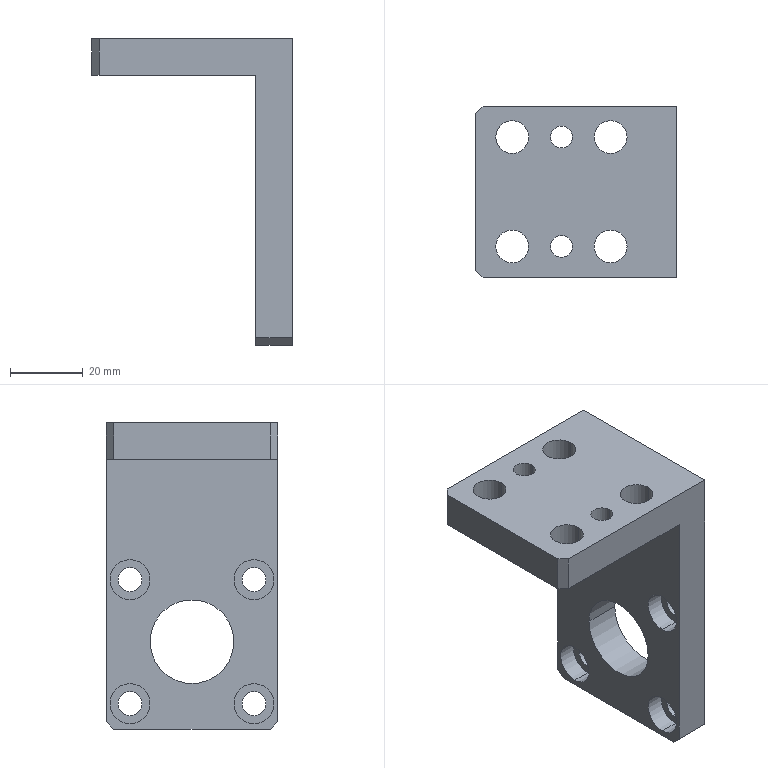Part | SolidWorks | features HoleWzd 3, Chamfer 2, ICE 2, CirPattern 1, Extrusion 1 | 1 solid | 46 faces | box 55 x 47 x 84 mm | volume 50700 mm3 | cylinder 30 | plane 16 | commonest cylinder face diameters 6.6 x8 9 x8 11 x8 6 x4 23 x2
STEP:
#1=CARTESIAN_POINT('',(22.5,-17.,-38.5));
#2=VERTEX_POINT('',#1);
#3=CARTESIAN_POINT('',(22.5,-17.,-27.5));
#4=VERTEX_POINT('',#3);
#5=CARTESIAN_POINT('',(22.5,-17.,-33.));
#6=DIRECTION('',(-1.,0.,0.));
#7=DIRECTION('',(0.,0.,1.));
#8=AXIS2_PLACEMENT_3D('',#5,#6,#7);
#9=CIRCLE('',#8,5.5);
#10=EDGE_CURVE('',#2,#4,#9,.T.);
#11=ORIENTED_EDGE('',*,*,#10,.F.);
#12=CARTESIAN_POINT('',(17.5,-17.,-38.5));
#13=VERTEX_POINT('',#12);
#14=CARTESIAN_POINT('',(17.5,-17.,-38.5));
#15=DIRECTION('',(-1.,0.,0.));
#16=VECTOR('',#15,1000.);
#17=LINE('',#14,#16);
#18=EDGE_CURVE('',#2,#13,#17,.T.);
#19=ORIENTED_EDGE('',*,*,#18,.T.);
#20=CARTESIAN_POINT('',(17.5,-17.,-27.5));
#21=VERTEX_POINT('',#20);
#22=CARTESIAN_POINT('',(17.5,-17.,-33.));
#23=DIRECTION('',(-1.,0.,0.));
#24=DIRECTION('',(0.,0.,1.));
#25=AXIS2_PLACEMENT_3D('',#22,#23,#24);
#26=CIRCLE('',#25,5.5);
#27=EDGE_CURVE('',#13,#21,#26,.T.);
#28=ORIENTED_EDGE('',*,*,#27,.T.);
#29=CARTESIAN_POINT('',(17.5,-17.,-27.5));
#30=DIRECTION('',(-1.,0.,0.));
#31=VECTOR('',#30,1000.);
#32=LINE('',#29,#31);
#33=EDGE_CURVE('',#4,#21,#32,.T.);
#34=ORIENTED_EDGE('',*,*,#33,.F.);
#35=EDGE_LOOP('',(#11,#19,#28,#34));
#36=FACE_OUTER_BOUND('',#35,.T.);
#37=CARTESIAN_POINT('',(17.5,-17.,-33.));
#38=DIRECTION('',(-1.,0.,0.));
#39=DIRECTION('',(0.,0.,1.));
#40=AXIS2_PLACEMENT_3D('',#37,#38,#39);
#41=CYLINDRICAL_SURFACE('',#40,5.5);
#42=ADVANCED_FACE('',(#36),#41,.F.);
#43=CARTESIAN_POINT('',(27.5,-17.,-36.3));
#44=VERTEX_POINT('',#43);
#45=CARTESIAN_POINT('',(27.5,-17.,-29.7));
#46=VERTEX_POINT('',#45);
#47=CARTESIAN_POINT('',(27.5,-17.,-33.));
#48=DIRECTION('',(-1.,0.,0.));
#49=DIRECTION('',(0.,-1.,0.));
#50=AXIS2_PLACEMENT_3D('',#47,#48,#49);
#51=CIRCLE('',#50,3.3);
#52=EDGE_CURVE('',#44,#46,#51,.T.);
#53=ORIENTED_EDGE('',*,*,#52,.F.);
#54=CARTESIAN_POINT('',(22.5,-17.,-36.3));
#55=VERTEX_POINT('',#54);
#56=CARTESIAN_POINT('',(17.5,-17.,-36.3));
#57=DIRECTION('',(-1.,0.,0.));
#58=VECTOR('',#57,1000.);
#59=LINE('',#56,#58);
#60=EDGE_CURVE('',#44,#55,#59,.T.);
#61=ORIENTED_EDGE('',*,*,#60,.T.);
#62=CARTESIAN_POINT('',(22.5,-17.,-29.7));
#63=VERTEX_POINT('',#62);
#64=CARTESIAN_POINT('',(22.5,-17.,-33.));
#65=DIRECTION('',(-1.,0.,0.));
#66=DIRECTION('',(0.,0.,1.));
#67=AXIS2_PLACEMENT_3D('',#64,#65,#66);
#68=CIRCLE('',#67,3.3);
#69=EDGE_CURVE('',#55,#63,#68,.T.);
#70=ORIENTED_EDGE('',*,*,#69,.T.);
#71=CARTESIAN_POINT('',(17.5,-17.,-29.7));
#72=DIRECTION('',(-1.,0.,0.));
#73=VECTOR('',#72,1000.);
#74=LINE('',#71,#73);
#75=EDGE_CURVE('',#46,#63,#74,.T.);
#76=ORIENTED_EDGE('',*,*,#75,.F.);
#77=EDGE_LOOP('',(#53,#61,#70,#76));
#78=FACE_OUTER_BOUND('',#77,.T.);
#79=CARTESIAN_POINT('',(17.5,-17.,-33.));
#80=DIRECTION('',(-1.,0.,0.));
#81=DIRECTION('',(0.,0.,1.));
#82=AXIS2_PLACEMENT_3D('',#79,#80,#81);
#83=CYLINDRICAL_SURFACE('',#82,3.3);
#84=ADVANCED_FACE('',(#78),#83,.F.);
#85=CARTESIAN_POINT('',(22.5,17.,-38.5));
#86=VERTEX_POINT('',#85);
#87=CARTESIAN_POINT('',(22.5,17.,-27.5));
#88=VERTEX_POINT('',#87);
#89=CARTESIAN_POINT('',(22.5,17.,-33.));
#90=DIRECTION('',(-1.,0.,0.));
#91=DIRECTION('',(0.,0.,1.));
#92=AXIS2_PLACEMENT_3D('',#89,#90,#91);
#93=CIRCLE('',#92,5.5);
#94=EDGE_CURVE('',#86,#88,#93,.T.);
#95=ORIENTED_EDGE('',*,*,#94,.F.);
#96=CARTESIAN_POINT('',(17.5,17.,-38.5));
#97=VERTEX_POINT('',#96);
#98=CARTESIAN_POINT('',(17.5,17.,-38.5));
#99=DIRECTION('',(-1.,0.,0.));
#100=VECTOR('',#99,1000.);
#101=LINE('',#98,#100);
#102=EDGE_CURVE('',#86,#97,#101,.T.);
#103=ORIENTED_EDGE('',*,*,#102,.T.);
#104=CARTESIAN_POINT('',(17.5,17.,-27.5));
#105=VERTEX_POINT('',#104);
#106=CARTESIAN_POINT('',(17.5,17.,-33.));
#107=DIRECTION('',(-1.,0.,0.));
#108=DIRECTION('',(0.,0.,1.));
#109=AXIS2_PLACEMENT_3D('',#106,#107,#108);
#110=CIRCLE('',#109,5.5);
#111=EDGE_CURVE('',#97,#105,#110,.T.);
#112=ORIENTED_EDGE('',*,*,#111,.T.);
#113=CARTESIAN_POINT('',(17.5,17.,-27.5));
#114=DIRECTION('',(-1.,0.,0.));
#115=VECTOR('',#114,1000.);
#116=LINE('',#113,#115);
#117=EDGE_CURVE('',#88,#105,#116,.T.);
#118=ORIENTED_EDGE('',*,*,#117,.F.);
#119=EDGE_LOOP('',(#95,#103,#112,#118));
#120=FACE_OUTER_BOUND('',#119,.T.);
#121=CARTESIAN_POINT('',(17.5,17.,-33.));
#122=DIRECTION('',(-1.,0.,0.));
#123=DIRECTION('',(0.,0.,1.));
#124=AXIS2_PLACEMENT_3D('',#121,#122,#123);
#125=CYLINDRICAL_SURFACE('',#124,5.5);
#126=ADVANCED_FACE('',(#120),#125,.F.);
#127=CARTESIAN_POINT('',(27.5,17.,-36.3));
#128=VERTEX_POINT('',#127);
#129=CARTESIAN_POINT('',(27.5,17.,-29.7));
#130=VERTEX_POINT('',#129);
#131=CARTESIAN_POINT('',(27.5,17.,-33.));
#132=DIRECTION('',(-1.,0.,0.));
#133=DIRECTION('',(0.,-1.,0.));
#134=AXIS2_PLACEMENT_3D('',#131,#132,#133);
#135=CIRCLE('',#134,3.3);
#136=EDGE_CURVE('',#128,#130,#135,.T.);
#137=ORIENTED_EDGE('',*,*,#136,.F.);
#138=CARTESIAN_POINT('',(22.5,17.,-36.3));
#139=VERTEX_POINT('',#138);
#140=CARTESIAN_POINT('',(17.5,17.,-36.3));
#141=DIRECTION('',(-1.,0.,0.));
#142=VECTOR('',#141,1000.);
#143=LINE('',#140,#142);
#144=EDGE_CURVE('',#128,#139,#143,.T.);
#145=ORIENTED_EDGE('',*,*,#144,.T.);
#146=CARTESIAN_POINT('',(22.5,17.,-29.7));
#147=VERTEX_POINT('',#146);
#148=CARTESIAN_POINT('',(22.5,17.,-33.));
#149=DIRECTION('',(-1.,0.,0.));
#150=DIRECTION('',(0.,0.,1.));
#151=AXIS2_PLACEMENT_3D('',#148,#149,#150);
#152=CIRCLE('',#151,3.3);
#153=EDGE_CURVE('',#139,#147,#152,.T.);
#154=ORIENTED_EDGE('',*,*,#153,.T.);
#155=CARTESIAN_POINT('',(17.5,17.,-29.7));
#156=DIRECTION('',(-1.,0.,0.));
#157=VECTOR('',#156,1000.);
#158=LINE('',#155,#157);
#159=EDGE_CURVE('',#130,#147,#158,.T.);
#160=ORIENTED_EDGE('',*,*,#159,.F.);
#161=EDGE_LOOP('',(#137,#145,#154,#160));
#162=FACE_OUTER_BOUND('',#161,.T.);
#163=CARTESIAN_POINT('',(17.5,17.,-33.));
#164=DIRECTION('',(-1.,0.,0.));
#165=DIRECTION('',(0.,0.,1.));
#166=AXIS2_PLACEMENT_3D('',#163,#164,#165);
#167=CYLINDRICAL_SURFACE('',#166,3.3);
#168=ADVANCED_FACE('',(#162),#167,.F.);
#169=CARTESIAN_POINT('',(22.5,17.,-72.5));
#170=VERTEX_POINT('',#169);
#171=CARTESIAN_POINT('',(22.5,17.,-61.5));
#172=VERTEX_POINT('',#171);
#173=CARTESIAN_POINT('',(22.5,17.,-67.));
#174=DIRECTION('',(-1.,0.,0.));
#175=DIRECTION('',(0.,0.,1.));
#176=AXIS2_PLACEMENT_3D('',#173,#174,#175);
#177=CIRCLE('',#176,5.5);
#178=EDGE_CURVE('',#170,#172,#177,.T.);
#179=ORIENTED_EDGE('',*,*,#178,.F.);
#180=CARTESIAN_POINT('',(17.5,17.,-72.5));
#181=VERTEX_POINT('',#180);
#182=CARTESIAN_POINT('',(17.5,17.,-72.5));
#183=DIRECTION('',(-1.,0.,0.));
#184=VECTOR('',#183,1000.);
#185=LINE('',#182,#184);
#186=EDGE_CURVE('',#170,#181,#185,.T.);
#187=ORIENTED_EDGE('',*,*,#186,.T.);
#188=CARTESIAN_POINT('',(17.5,17.,-61.5));
#189=VERTEX_POINT('',#188);
#190=CARTESIAN_POINT('',(17.5,17.,-67.));
#191=DIRECTION('',(-1.,0.,0.));
#192=DIRECTION('',(0.,0.,1.));
#193=AXIS2_PLACEMENT_3D('',#190,#191,#192);
#194=CIRCLE('',#193,5.5);
#195=EDGE_CURVE('',#181,#189,#194,.T.);
#196=ORIENTED_EDGE('',*,*,#195,.T.);
#197=CARTESIAN_POINT('',(17.5,17.,-61.5));
#198=DIRECTION('',(-1.,0.,0.));
#199=VECTOR('',#198,1000.);
#200=LINE('',#197,#199);
#201=EDGE_CURVE('',#172,#189,#200,.T.);
#202=ORIENTED_EDGE('',*,*,#201,.F.);
#203=EDGE_LOOP('',(#179,#187,#196,#202));
#204=FACE_OUTER_BOUND('',#203,.T.);
#205=CARTESIAN_POINT('',(17.5,17.,-67.));
#206=DIRECTION('',(-1.,0.,0.));
#207=DIRECTION('',(0.,0.,1.));
#208=AXIS2_PLACEMENT_3D('',#205,#206,#207);
#209=CYLINDRICAL_SURFACE('',#208,5.5);
#210=ADVANCED_FACE('',(#204),#209,.F.);
#211=CARTESIAN_POINT('',(27.5,17.,-70.3));
#212=VERTEX_POINT('',#211);
#213=CARTESIAN_POINT('',(27.5,17.,-63.7));
#214=VERTEX_POINT('',#213);
#215=CARTESIAN_POINT('',(27.5,17.,-67.));
#216=DIRECTION('',(-1.,0.,0.));
#217=DIRECTION('',(0.,-1.,0.));
#218=AXIS2_PLACEMENT_3D('',#215,#216,#217);
#219=CIRCLE('',#218,3.3);
#220=EDGE_CURVE('',#212,#214,#219,.T.);
#221=ORIENTED_EDGE('',*,*,#220,.F.);
#222=CARTESIAN_POINT('',(22.5,17.,-70.3));
#223=VERTEX_POINT('',#222);
#224=CARTESIAN_POINT('',(17.5,17.,-70.3));
#225=DIRECTION('',(-1.,0.,0.));
#226=VECTOR('',#225,1000.);
#227=LINE('',#224,#226);
#228=EDGE_CURVE('',#212,#223,#227,.T.);
#229=ORIENTED_EDGE('',*,*,#228,.T.);
#230=CARTESIAN_POINT('',(22.5,17.,-63.7));
#231=VERTEX_POINT('',#230);
#232=CARTESIAN_POINT('',(22.5,17.,-67.));
#233=DIRECTION('',(-1.,0.,0.));
#234=DIRECTION('',(0.,0.,1.));
#235=AXIS2_PLACEMENT_3D('',#232,#233,#234);
#236=CIRCLE('',#235,3.3);
#237=EDGE_CURVE('',#223,#231,#236,.T.);
#238=ORIENTED_EDGE('',*,*,#237,.T.);
#239=CARTESIAN_POINT('',(17.5,17.,-63.7));
#240=DIRECTION('',(-1.,0.,0.));
#241=VECTOR('',#240,1000.);
#242=LINE('',#239,#241);
#243=EDGE_CURVE('',#214,#231,#242,.T.);
#244=ORIENTED_EDGE('',*,*,#243,.F.);
#245=EDGE_LOOP('',(#221,#229,#238,#244));
#246=FACE_OUTER_BOUND('',#245,.T.);
#247=CARTESIAN_POINT('',(17.5,17.,-67.));
#248=DIRECTION('',(-1.,0.,0.));
#249=DIRECTION('',(0.,0.,1.));
#250=AXIS2_PLACEMENT_3D('',#247,#248,#249);
#251=CYLINDRICAL_SURFACE('',#250,3.3);
#252=ADVANCED_FACE('',(#246),#251,.F.);
#253=CARTESIAN_POINT('',(22.5,-17.,-72.5));
#254=VERTEX_POINT('',#253);
#255=CARTESIAN_POINT('',(22.5,-17.,-61.5));
#256=VERTEX_POINT('',#255);
#257=CARTESIAN_POINT('',(22.5,-17.,-67.));
#258=DIRECTION('',(-1.,0.,0.));
#259=DIRECTION('',(0.,0.,1.));
#260=AXIS2_PLACEMENT_3D('',#257,#258,#259);
#261=CIRCLE('',#260,5.5);
#262=EDGE_CURVE('',#254,#256,#261,.T.);
#263=ORIENTED_EDGE('',*,*,#262,.F.);
#264=CARTESIAN_POINT('',(17.5,-17.,-72.5));
#265=VERTEX_POINT('',#264);
#266=CARTESIAN_POINT('',(17.5,-17.,-72.5));
#267=DIRECTION('',(-1.,0.,0.));
#268=VECTOR('',#267,1000.);
#269=LINE('',#266,#268);
#270=EDGE_CURVE('',#254,#265,#269,.T.);
#271=ORIENTED_EDGE('',*,*,#270,.T.);
#272=CARTESIAN_POINT('',(17.5,-17.,-61.5));
#273=VERTEX_POINT('',#272);
#274=CARTESIAN_POINT('',(17.5,-17.,-67.));
#275=DIRECTION('',(-1.,0.,0.));
#276=DIRECTION('',(0.,0.,1.));
#277=AXIS2_PLACEMENT_3D('',#274,#275,#276);
#278=CIRCLE('',#277,5.5);
#279=EDGE_CURVE('',#265,#273,#278,.T.);
#280=ORIENTED_EDGE('',*,*,#279,.T.);
#281=CARTESIAN_POINT('',(17.5,-17.,-61.5));
#282=DIRECTION('',(-1.,0.,0.));
#283=VECTOR('',#282,1000.);
#284=LINE('',#281,#283);
#285=EDGE_CURVE('',#256,#273,#284,.T.);
#286=ORIENTED_EDGE('',*,*,#285,.F.);
#287=EDGE_LOOP('',(#263,#271,#280,#286));
#288=FACE_OUTER_BOUND('',#287,.T.);
#289=CARTESIAN_POINT('',(17.5,-17.,-67.));
#290=DIRECTION('',(-1.,0.,0.));
#291=DIRECTION('',(0.,0.,1.));
#292=AXIS2_PLACEMENT_3D('',#289,#290,#291);
#293=CYLINDRICAL_SURFACE('',#292,5.5);
#294=ADVANCED_FACE('',(#288),#293,.F.);
#295=CARTESIAN_POINT('',(27.5,-17.,-70.3));
#296=VERTEX_POINT('',#295);
#297=CARTESIAN_POINT('',(27.5,-17.,-63.7));
#298=VERTEX_POINT('',#297);
#299=CARTESIAN_POINT('',(27.5,-17.,-67.));
#300=DIRECTION('',(-1.,0.,0.));
#301=DIRECTION('',(0.,-1.,0.));
#302=AXIS2_PLACEMENT_3D('',#299,#300,#301);
#303=CIRCLE('',#302,3.3);
#304=EDGE_CURVE('',#296,#298,#303,.T.);
#305=ORIENTED_EDGE('',*,*,#304,.F.);
#306=CARTESIAN_POINT('',(22.5,-17.,-70.3));
#307=VERTEX_POINT('',#306);
#308=CARTESIAN_POINT('',(17.5,-17.,-70.3));
#309=DIRECTION('',(-1.,0.,0.));
#310=VECTOR('',#309,1000.);
#311=LINE('',#308,#310);
#312=EDGE_CURVE('',#296,#307,#311,.T.);
#313=ORIENTED_EDGE('',*,*,#312,.T.);
#314=CARTESIAN_POINT('',(22.5,-17.,-63.7));
#315=VERTEX_POINT('',#314);
#316=CARTESIAN_POINT('',(22.5,-17.,-67.));
#317=DIRECTION('',(-1.,0.,0.));
#318=DIRECTION('',(0.,0.,1.));
#319=AXIS2_PLACEMENT_3D('',#316,#317,#318);
#320=CIRCLE('',#319,3.3);
#321=EDGE_CURVE('',#307,#315,#320,.T.);
#322=ORIENTED_EDGE('',*,*,#321,.T.);
#323=CARTESIAN_POINT('',(17.5,-17.,-63.7));
#324=DIRECTION('',(-1.,0.,0.));
#325=VECTOR('',#324,1000.);
#326=LINE('',#323,#325);
#327=EDGE_CURVE('',#298,#315,#326,.T.);
#328=ORIENTED_EDGE('',*,*,#327,.F.);
#329=EDGE_LOOP('',(#305,#313,#322,#328));
#330=FACE_OUTER_BOUND('',#329,.T.);
#331=CARTESIAN_POINT('',(17.5,-17.,-67.));
#332=DIRECTION('',(-1.,0.,0.));
#333=DIRECTION('',(0.,0.,1.));
#334=AXIS2_PLACEMENT_3D('',#331,#332,#333);
#335=CYLINDRICAL_SURFACE('',#334,3.3);
#336=ADVANCED_FACE('',(#330),#335,.F.);
#337=CARTESIAN_POINT('',(-1.,-15.,10.));
#338=VERTEX_POINT('',#337);
#339=CARTESIAN_POINT('',(-7.,-15.,10.));
#340=VERTEX_POINT('',#339);
#341=CARTESIAN_POINT('',(-4.,-15.,10.));
#342=DIRECTION('',(0.,0.,-1.));
#343=DIRECTION('',(-1.,0.,0.));
#344=AXIS2_PLACEMENT_3D('',#341,#342,#343);
#345=CIRCLE('',#344,3.);
#346=EDGE_CURVE('',#338,#340,#345,.T.);
#347=ORIENTED_EDGE('',*,*,#346,.F.);
#348=CARTESIAN_POINT('',(-1.,-15.,0.));
#349=VERTEX_POINT('',#348);
#350=CARTESIAN_POINT('',(-1.,-15.,0.));
#351=DIRECTION('',(0.,0.,-1.));
#352=VECTOR('',#351,1000.);
#353=LINE('',#350,#352);
#354=EDGE_CURVE('',#338,#349,#353,.T.);
#355=ORIENTED_EDGE('',*,*,#354,.T.);
#356=CARTESIAN_POINT('',(-7.,-15.,0.));
#357=VERTEX_POINT('',#356);
#358=CARTESIAN_POINT('',(-4.,-15.,0.));
#359=DIRECTION('',(0.,0.,-1.));
#360=DIRECTION('',(-1.,0.,0.));
#361=AXIS2_PLACEMENT_3D('',#358,#359,#360);
#362=CIRCLE('',#361,3.);
#363=EDGE_CURVE('',#349,#357,#362,.T.);
#364=ORIENTED_EDGE('',*,*,#363,.T.);
#365=CARTESIAN_POINT('',(-7.,-15.,0.));
#366=DIRECTION('',(0.,0.,-1.));
#367=VECTOR('',#366,1000.);
#368=LINE('',#365,#367);
#369=EDGE_CURVE('',#340,#357,#368,.T.);
#370=ORIENTED_EDGE('',*,*,#369,.F.);
#371=EDGE_LOOP('',(#347,#355,#364,#370));
#372=FACE_OUTER_BOUND('',#371,.T.);
#373=CARTESIAN_POINT('',(-4.,-15.,0.));
#374=DIRECTION('',(0.,0.,-1.));
#375=DIRECTION('',(-1.,0.,0.));
#376=AXIS2_PLACEMENT_3D('',#373,#374,#375);
#377=CYLINDRICAL_SURFACE('',#376,3.);
#378=ADVANCED_FACE('',(#372),#377,.F.);
#379=CARTESIAN_POINT('',(-1.,15.,10.));
#380=VERTEX_POINT('',#379);
#381=CARTESIAN_POINT('',(-7.,15.,10.));
#382=VERTEX_POINT('',#381);
#383=CARTESIAN_POINT('',(-4.,15.,10.));
#384=DIRECTION('',(0.,0.,-1.));
#385=DIRECTION('',(-1.,0.,0.));
#386=AXIS2_PLACEMENT_3D('',#383,#384,#385);
#387=CIRCLE('',#386,3.);
#388=EDGE_CURVE('',#380,#382,#387,.T.);
#389=ORIENTED_EDGE('',*,*,#388,.F.);
#390=CARTESIAN_POINT('',(-1.,15.,0.));
#391=VERTEX_POINT('',#390);
#392=CARTESIAN_POINT('',(-1.,15.,0.));
#393=DIRECTION('',(0.,0.,-1.));
#394=VECTOR('',#393,1000.);
#395=LINE('',#392,#394);
#396=EDGE_CURVE('',#380,#391,#395,.T.);
#397=ORIENTED_EDGE('',*,*,#396,.T.);
#398=CARTESIAN_POINT('',(-7.,15.,0.));
#399=VERTEX_POINT('',#398);
#400=CARTESIAN_POINT('',(-4.,15.,0.));
#401=DIRECTION('',(0.,0.,-1.));
#402=DIRECTION('',(-1.,0.,0.));
#403=AXIS2_PLACEMENT_3D('',#400,#401,#402);
#404=CIRCLE('',#403,3.);
#405=EDGE_CURVE('',#391,#399,#404,.T.);
#406=ORIENTED_EDGE('',*,*,#405,.T.);
#407=CARTESIAN_POINT('',(-7.,15.,0.));
#408=DIRECTION('',(0.,0.,-1.));
#409=VECTOR('',#408,1000.);
#410=LINE('',#407,#409);
#411=EDGE_CURVE('',#382,#399,#410,.T.);
#412=ORIENTED_EDGE('',*,*,#411,.F.);
#413=EDGE_LOOP('',(#389,#397,#406,#412));
#414=FACE_OUTER_BOUND('',#413,.T.);
#415=CARTESIAN_POINT('',(-4.,15.,0.));
#416=DIRECTION('',(0.,0.,-1.));
#417=DIRECTION('',(-1.,0.,0.));
#418=AXIS2_PLACEMENT_3D('',#415,#416,#417);
#419=CYLINDRICAL_SURFACE('',#418,3.);
#420=ADVANCED_FACE('',(#414),#419,.F.);
#421=CARTESIAN_POINT('',(27.5,11.5,-50.));
#422=VERTEX_POINT('',#421);
#423=CARTESIAN_POINT('',(27.5,-11.5,-50.));
#424=VERTEX_POINT('',#423);
#425=CARTESIAN_POINT('',(27.5,0.,-50.));
#426=DIRECTION('',(-1.,0.,0.));
#427=DIRECTION('',(0.,-1.,0.));
#428=AXIS2_PLACEMENT_3D('',#425,#426,#427);
#429=CIRCLE('',#428,11.5);
#430=EDGE_CURVE('',#422,#424,#429,.T.);
#431=ORIENTED_EDGE('',*,*,#430,.F.);
#432=CARTESIAN_POINT('',(17.5,11.5,-50.));
#433=VERTEX_POINT('',#432);
#434=CARTESIAN_POINT('',(47.5,11.5,-50.));
#435=DIRECTION('',(-1.,0.,0.));
#436=VECTOR('',#435,1000.);
#437=LINE('',#434,#436);
#438=EDGE_CURVE('',#422,#433,#437,.T.);
#439=ORIENTED_EDGE('',*,*,#438,.T.);
#440=CARTESIAN_POINT('',(17.5,-11.5,-50.));
#441=VERTEX_POINT('',#440);
#442=CARTESIAN_POINT('',(17.5,0.,-50.));
#443=DIRECTION('',(-1.,0.,0.));
#444=DIRECTION('',(0.,-1.,0.));
#445=AXIS2_PLACEMENT_3D('',#442,#443,#444);
#446=CIRCLE('',#445,11.5);
#447=EDGE_CURVE('',#433,#441,#446,.T.);
#448=ORIENTED_EDGE('',*,*,#447,.T.);
#449=CARTESIAN_POINT('',(47.5,-11.5,-50.));
#450=DIRECTION('',(-1.,0.,0.));
#451=VECTOR('',#450,1000.);
#452=LINE('',#449,#451);
#453=EDGE_CURVE('',#424,#441,#452,.T.);
#454=ORIENTED_EDGE('',*,*,#453,.F.);
#455=EDGE_LOOP('',(#431,#439,#448,#454));
#456=FACE_OUTER_BOUND('',#455,.T.);
#457=CARTESIAN_POINT('',(47.5,0.,-50.));
#458=DIRECTION('',(-1.,0.,0.));
#459=DIRECTION('',(0.,-1.,0.));
#460=AXIS2_PLACEMENT_3D('',#457,#458,#459);
#461=CYLINDRICAL_SURFACE('',#460,11.5);
#462=ADVANCED_FACE('',(#456),#461,.F.);
#463=CARTESIAN_POINT('',(-22.,-15.,10.));
#464=VERTEX_POINT('',#463);
#465=CARTESIAN_POINT('',(-13.,-15.,10.));
#466=VERTEX_POINT('',#465);
#467=CARTESIAN_POINT('',(-17.5,-15.,10.));
#468=DIRECTION('',(0.,0.,1.));
#469=DIRECTION('',(1.,0.,0.));
#470=AXIS2_PLACEMENT_3D('',#467,#468,#469);
#471=CIRCLE('',#470,4.5);
#472=EDGE_CURVE('',#464,#466,#471,.T.);
#473=ORIENTED_EDGE('',*,*,#472,.T.);
#474=CARTESIAN_POINT('',(-13.,-15.,0.));
#475=VERTEX_POINT('',#474);
#476=CARTESIAN_POINT('',(-13.,-15.,0.));
#477=DIRECTION('',(0.,0.,-1.));
#478=VECTOR('',#477,1000.);
#479=LINE('',#476,#478);
#480=EDGE_CURVE('',#466,#475,#479,.T.);
#481=ORIENTED_EDGE('',*,*,#480,.T.);
#482=CARTESIAN_POINT('',(-22.,-15.,0.));
#483=VERTEX_POINT('',#482);
#484=CARTESIAN_POINT('',(-17.5,-15.,0.));
#485=DIRECTION('',(0.,0.,-1.));
#486=DIRECTION('',(-1.,0.,0.));
#487=AXIS2_PLACEMENT_3D('',#484,#485,#486);
#488=CIRCLE('',#487,4.5);
#489=EDGE_CURVE('',#475,#483,#488,.T.);
#490=ORIENTED_EDGE('',*,*,#489,.T.);
#491=CARTESIAN_POINT('',(-22.,-15.,0.));
#492=DIRECTION('',(0.,0.,-1.));
#493=VECTOR('',#492,1000.);
#494=LINE('',#491,#493);
#495=EDGE_CURVE('',#464,#483,#494,.T.);
#496=ORIENTED_EDGE('',*,*,#495,.F.);
#497=EDGE_LOOP('',(#473,#481,#490,#496));
#498=FACE_OUTER_BOUND('',#497,.T.);
#499=CARTESIAN_POINT('',(-17.5,-15.,0.));
#500=DIRECTION('',(0.,0.,-1.));
#501=DIRECTION('',(-1.,0.,0.));
#502=AXIS2_PLACEMENT_3D('',#499,#500,#501);
#503=CYLINDRICAL_SURFACE('',#502,4.5);
#504=ADVANCED_FACE('',(#498),#503,.F.);
#505=CARTESIAN_POINT('',(-22.,15.,10.));
#506=VERTEX_POINT('',#505);
#507=CARTESIAN_POINT('',(-13.,15.,10.));
#508=VERTEX_POINT('',#507);
#509=CARTESIAN_POINT('',(-17.5,15.,10.));
#510=DIRECTION('',(0.,0.,1.));
#511=DIRECTION('',(1.,0.,0.));
#512=AXIS2_PLACEMENT_3D('',#509,#510,#511);
#513=CIRCLE('',#512,4.5);
#514=EDGE_CURVE('',#506,#508,#513,.T.);
#515=ORIENTED_EDGE('',*,*,#514,.T.);
#516=CARTESIAN_POINT('',(-13.,15.,0.));
#517=VERTEX_POINT('',#516);
#518=CARTESIAN_POINT('',(-13.,15.,0.));
#519=DIRECTION('',(0.,0.,-1.));
#520=VECTOR('',#519,1000.);
#521=LINE('',#518,#520);
#522=EDGE_CURVE('',#508,#517,#521,.T.);
#523=ORIENTED_EDGE('',*,*,#522,.T.);
#524=CARTESIAN_POINT('',(-22.,15.,0.));
#525=VERTEX_POINT('',#524);
#526=CARTESIAN_POINT('',(-17.5,15.,0.));
#527=DIRECTION('',(0.,0.,-1.));
#528=DIRECTION('',(-1.,0.,0.));
#529=AXIS2_PLACEMENT_3D('',#526,#527,#528);
#530=CIRCLE('',#529,4.5);
#531=EDGE_CURVE('',#517,#525,#530,.T.);
#532=ORIENTED_EDGE('',*,*,#531,.T.);
#533=CARTESIAN_POINT('',(-22.,15.,0.));
#534=DIRECTION('',(0.,0.,-1.));
#535=VECTOR('',#534,1000.);
#536=LINE('',#533,#535);
#537=EDGE_CURVE('',#506,#525,#536,.T.);
#538=ORIENTED_EDGE('',*,*,#537,.F.);
#539=EDGE_LOOP('',(#515,#523,#532,#538));
#540=FACE_OUTER_BOUND('',#539,.T.);
#541=CARTESIAN_POINT('',(-17.5,15.,0.));
#542=DIRECTION('',(0.,0.,-1.));
#543=DIRECTION('',(-1.,0.,0.));
#544=AXIS2_PLACEMENT_3D('',#541,#542,#543);
#545=CYLINDRICAL_SURFACE('',#544,4.5);
#546=ADVANCED_FACE('',(#540),#545,.F.);
#547=CARTESIAN_POINT('',(5.,-15.,10.));
#548=VERTEX_POINT('',#547);
#549=CARTESIAN_POINT('',(14.,-15.,10.));
#550=VERTEX_POINT('',#549);
#551=CARTESIAN_POINT('',(9.5,-15.,10.));
#552=DIRECTION('',(0.,0.,1.));
#553=DIRECTION('',(1.,0.,0.));
#554=AXIS2_PLACEMENT_3D('',#551,#552,#553);
#555=CIRCLE('',#554,4.5);
#556=EDGE_CURVE('',#548,#550,#555,.T.);
#557=ORIENTED_EDGE('',*,*,#556,.T.);
#558=CARTESIAN_POINT('',(14.,-15.,0.));
#559=VERTEX_POINT('',#558);
#560=CARTESIAN_POINT('',(14.,-15.,0.));
#561=DIRECTION('',(0.,0.,-1.));
#562=VECTOR('',#561,1000.);
#563=LINE('',#560,#562);
#564=EDGE_CURVE('',#550,#559,#563,.T.);
#565=ORIENTED_EDGE('',*,*,#564,.T.);
#566=CARTESIAN_POINT('',(5.,-15.,0.));
#567=VERTEX_POINT('',#566);
#568=CARTESIAN_POINT('',(9.5,-15.,0.));
#569=DIRECTION('',(0.,0.,-1.));
#570=DIRECTION('',(-1.,0.,0.));
#571=AXIS2_PLACEMENT_3D('',#568,#569,#570);
#572=CIRCLE('',#571,4.5);
#573=EDGE_CURVE('',#559,#567,#572,.T.);
#574=ORIENTED_EDGE('',*,*,#573,.T.);
#575=CARTESIAN_POINT('',(5.,-15.,0.));
#576=DIRECTION('',(0.,0.,-1.));
#577=VECTOR('',#576,1000.);
#578=LINE('',#575,#577);
#579=EDGE_CURVE('',#548,#567,#578,.T.);
#580=ORIENTED_EDGE('',*,*,#579,.F.);
#581=EDGE_LOOP('',(#557,#565,#574,#580));
#582=FACE_OUTER_BOUND('',#581,.T.);
#583=CARTESIAN_POINT('',(9.5,-15.,0.));
#584=DIRECTION('',(0.,0.,-1.));
#585=DIRECTION('',(-1.,0.,0.));
#586=AXIS2_PLACEMENT_3D('',#583,#584,#585);
#587=CYLINDRICAL_SURFACE('',#586,4.5);
#588=ADVANCED_FACE('',(#582),#587,.F.);
#589=CARTESIAN_POINT('',(5.,15.,10.));
#590=VERTEX_POINT('',#589);
#591=CARTESIAN_POINT('',(14.,15.,10.));
#592=VERTEX_POINT('',#591);
#593=CARTESIAN_POINT('',(9.5,15.,10.));
#594=DIRECTION('',(0.,0.,1.));
#595=DIRECTION('',(1.,0.,0.));
#596=AXIS2_PLACEMENT_3D('',#593,#594,#595);
#597=CIRCLE('',#596,4.5);
#598=EDGE_CURVE('',#590,#592,#597,.T.);
#599=ORIENTED_EDGE('',*,*,#598,.T.);
#600=CARTESIAN_POINT('',(14.,15.,0.));
#601=VERTEX_POINT('',#600);
#602=CARTESIAN_POINT('',(14.,15.,0.));
#603=DIRECTION('',(0.,0.,-1.));
#604=VECTOR('',#603,1000.);
#605=LINE('',#602,#604);
#606=EDGE_CURVE('',#592,#601,#605,.T.);
#607=ORIENTED_EDGE('',*,*,#606,.T.);
#608=CARTESIAN_POINT('',(5.,15.,0.));
#609=VERTEX_POINT('',#608);
#610=CARTESIAN_POINT('',(9.5,15.,0.));
#611=DIRECTION('',(0.,0.,-1.));
#612=DIRECTION('',(-1.,0.,0.));
#613=AXIS2_PLACEMENT_3D('',#610,#611,#612);
#614=CIRCLE('',#613,4.5);
#615=EDGE_CURVE('',#601,#609,#614,.T.);
#616=ORIENTED_EDGE('',*,*,#615,.T.);
#617=CARTESIAN_POINT('',(5.,15.,0.));
#618=DIRECTION('',(0.,0.,-1.));
#619=VECTOR('',#618,1000.);
#620=LINE('',#617,#619);
#621=EDGE_CURVE('',#590,#609,#620,.T.);
#622=ORIENTED_EDGE('',*,*,#621,.F.);
#623=EDGE_LOOP('',(#599,#607,#616,#622));
#624=FACE_OUTER_BOUND('',#623,.T.);
#625=CARTESIAN_POINT('',(9.5,15.,0.));
#626=DIRECTION('',(0.,0.,-1.));
#627=DIRECTION('',(-1.,0.,0.));
#628=AXIS2_PLACEMENT_3D('',#625,#626,#627);
#629=CYLINDRICAL_SURFACE('',#628,4.5);
#630=ADVANCED_FACE('',(#624),#629,.F.);
#631=CARTESIAN_POINT('',(-4.,-15.,0.));
#632=DIRECTION('',(0.,0.,-1.));
#633=DIRECTION('',(-1.,0.,0.));
#634=AXIS2_PLACEMENT_3D('',#631,#632,#633);
#635=CIRCLE('',#634,3.);
#636=EDGE_CURVE('',#357,#349,#635,.T.);
#637=ORIENTED_EDGE('',*,*,#636,.F.);
#638=ORIENTED_EDGE('',*,*,#363,.F.);
#639=EDGE_LOOP('',(#637,#638));
#640=FACE_BOUND('',#639,.T.);
#641=CARTESIAN_POINT('',(-4.,15.,0.));
#642=DIRECTION('',(0.,0.,-1.));
#643=DIRECTION('',(-1.,0.,0.));
#644=AXIS2_PLACEMENT_3D('',#641,#642,#643);
#645=CIRCLE('',#644,3.);
#646=EDGE_CURVE('',#399,#391,#645,.T.);
#647=ORIENTED_EDGE('',*,*,#646,.F.);
#648=ORIENTED_EDGE('',*,*,#405,.F.);
#649=EDGE_LOOP('',(#647,#648));
#650=FACE_BOUND('',#649,.T.);
#651=CARTESIAN_POINT('',(-17.5,-15.,0.));
#652=DIRECTION('',(0.,0.,-1.));
#653=DIRECTION('',(-1.,0.,0.));
#654=AXIS2_PLACEMENT_3D('',#651,#652,#653);
#655=CIRCLE('',#654,4.5);
#656=EDGE_CURVE('',#483,#475,#655,.T.);
#657=ORIENTED_EDGE('',*,*,#656,.F.);
#658=ORIENTED_EDGE('',*,*,#489,.F.);
#659=EDGE_LOOP('',(#657,#658));
#660=FACE_BOUND('',#659,.T.);
#661=CARTESIAN_POINT('',(-17.5,15.,0.));
#662=DIRECTION('',(0.,0.,-1.));
#663=DIRECTION('',(-1.,0.,0.));
#664=AXIS2_PLACEMENT_3D('',#661,#662,#663);
#665=CIRCLE('',#664,4.5);
#666=EDGE_CURVE('',#525,#517,#665,.T.);
#667=ORIENTED_EDGE('',*,*,#666,.F.);
#668=ORIENTED_EDGE('',*,*,#531,.F.);
#669=EDGE_LOOP('',(#667,#668));
#670=FACE_BOUND('',#669,.T.);
#671=CARTESIAN_POINT('',(9.5,-15.,0.));
#672=DIRECTION('',(0.,0.,-1.));
#673=DIRECTION('',(-1.,0.,0.));
#674=AXIS2_PLACEMENT_3D('',#671,#672,#673);
#675=CIRCLE('',#674,4.5);
#676=EDGE_CURVE('',#567,#559,#675,.T.);
#677=ORIENTED_EDGE('',*,*,#676,.F.);
#678=ORIENTED_EDGE('',*,*,#573,.F.);
#679=EDGE_LOOP('',(#677,#678));
#680=FACE_BOUND('',#679,.T.);
#681=CARTESIAN_POINT('',(9.5,15.,0.));
#682=DIRECTION('',(0.,0.,-1.));
#683=DIRECTION('',(-1.,0.,0.));
#684=AXIS2_PLACEMENT_3D('',#681,#682,#683);
#685=CIRCLE('',#684,4.5);
#686=EDGE_CURVE('',#609,#601,#685,.T.);
#687=ORIENTED_EDGE('',*,*,#686,.F.);
#688=ORIENTED_EDGE('',*,*,#615,.F.);
#689=EDGE_LOOP('',(#687,#688));
#690=FACE_BOUND('',#689,.T.);
#691=CARTESIAN_POINT('',(-25.5,-23.5,0.));
#692=VERTEX_POINT('',#691);
#693=CARTESIAN_POINT('',(17.5,-23.5,0.));
#694=VERTEX_POINT('',#693);
#695=CARTESIAN_POINT('',(-27.5,-23.5,0.));
#696=DIRECTION('',(1.,0.,0.));
#697=VECTOR('',#696,1000.);
#698=LINE('',#695,#697);
#699=EDGE_CURVE('',#692,#694,#698,.T.);
#700=ORIENTED_EDGE('',*,*,#699,.F.);
#701=CARTESIAN_POINT('',(-27.5,-21.5,0.));
#702=VERTEX_POINT('',#701);
#703=CARTESIAN_POINT('',(-25.5,-23.5,0.));
#704=DIRECTION('',(-0.7071,0.7071,0.));
#705=VECTOR('',#704,1000.);
#706=LINE('',#703,#705);
#707=EDGE_CURVE('',#692,#702,#706,.T.);
#708=ORIENTED_EDGE('',*,*,#707,.T.);
#709=CARTESIAN_POINT('',(-27.5,21.5,0.));
#710=VERTEX_POINT('',#709);
#711=CARTESIAN_POINT('',(-27.5,23.5,0.));
#712=DIRECTION('',(0.,-1.,0.));
#713=VECTOR('',#712,1000.);
#714=LINE('',#711,#713);
#715=EDGE_CURVE('',#710,#702,#714,.T.);
#716=ORIENTED_EDGE('',*,*,#715,.F.);
#717=CARTESIAN_POINT('',(-25.5,23.5,0.));
#718=VERTEX_POINT('',#717);
#719=CARTESIAN_POINT('',(-27.5,21.5,0.));
#720=DIRECTION('',(0.7071,0.7071,0.));
#721=VECTOR('',#720,1000.);
#722=LINE('',#719,#721);
#723=EDGE_CURVE('',#710,#718,#722,.T.);
#724=ORIENTED_EDGE('',*,*,#723,.T.);
#725=CARTESIAN_POINT('',(17.5,23.5,0.));
#726=VERTEX_POINT('',#725);
#727=CARTESIAN_POINT('',(-27.5,23.5,0.));
#728=DIRECTION('',(-1.,0.,0.));
#729=VECTOR('',#728,1000.);
#730=LINE('',#727,#729);
#731=EDGE_CURVE('',#726,#718,#730,.T.);
#732=ORIENTED_EDGE('',*,*,#731,.F.);
#733=CARTESIAN_POINT('',(17.5,23.5,0.));
#734=DIRECTION('',(0.,1.,0.));
#735=VECTOR('',#734,1000.);
#736=LINE('',#733,#735);
#737=EDGE_CURVE('',#694,#726,#736,.T.);
#738=ORIENTED_EDGE('',*,*,#737,.F.);
#739=EDGE_LOOP('',(#700,#708,#716,#724,#732,#738));
#740=FACE_OUTER_BOUND('',#739,.T.);
#741=CARTESIAN_POINT('',(0.,0.,0.));
#742=DIRECTION('',(0.,0.,1.));
#743=DIRECTION('',(1.,0.,0.));
#744=AXIS2_PLACEMENT_3D('',#741,#742,#743);
#745=PLANE('',#744);
#746=ADVANCED_FACE('',(#640,#650,#660,#670,#680,#690,#740),#745,.F.);
#747=CARTESIAN_POINT('',(27.5,-17.,-33.));
#748=DIRECTION('',(-1.,0.,0.));
#749=DIRECTION('',(0.,-1.,0.));
#750=AXIS2_PLACEMENT_3D('',#747,#748,#749);
#751=CIRCLE('',#750,3.3);
#752=EDGE_CURVE('',#46,#44,#751,.T.);
#753=ORIENTED_EDGE('',*,*,#752,.T.);
#754=ORIENTED_EDGE('',*,*,#52,.T.);
#755=EDGE_LOOP('',(#753,#754));
#756=FACE_BOUND('',#755,.T.);
#757=CARTESIAN_POINT('',(27.5,17.,-33.));
#758=DIRECTION('',(-1.,0.,0.));
#759=DIRECTION('',(0.,-1.,0.));
#760=AXIS2_PLACEMENT_3D('',#757,#758,#759);
#761=CIRCLE('',#760,3.3);
#762=EDGE_CURVE('',#130,#128,#761,.T.);
#763=ORIENTED_EDGE('',*,*,#762,.T.);
#764=ORIENTED_EDGE('',*,*,#136,.T.);
#765=EDGE_LOOP('',(#763,#764));
#766=FACE_BOUND('',#765,.T.);
#767=CARTESIAN_POINT('',(27.5,17.,-67.));
#768=DIRECTION('',(-1.,0.,0.));
#769=DIRECTION('',(0.,-1.,0.));
#770=AXIS2_PLACEMENT_3D('',#767,#768,#769);
#771=CIRCLE('',#770,3.3);
#772=EDGE_CURVE('',#214,#212,#771,.T.);
#773=ORIENTED_EDGE('',*,*,#772,.T.);
#774=ORIENTED_EDGE('',*,*,#220,.T.);
#775=EDGE_LOOP('',(#773,#774));
#776=FACE_BOUND('',#775,.T.);
#777=CARTESIAN_POINT('',(27.5,-17.,-67.));
#778=DIRECTION('',(-1.,0.,0.));
#779=DIRECTION('',(0.,-1.,0.));
#780=AXIS2_PLACEMENT_3D('',#777,#778,#779);
#781=CIRCLE('',#780,3.3);
#782=EDGE_CURVE('',#298,#296,#781,.T.);
#783=ORIENTED_EDGE('',*,*,#782,.T.);
#784=ORIENTED_EDGE('',*,*,#304,.T.);
#785=EDGE_LOOP('',(#783,#784));
#786=FACE_BOUND('',#785,.T.);
#787=CARTESIAN_POINT('',(27.5,0.,-50.));
#788=DIRECTION('',(-1.,0.,0.));
#789=DIRECTION('',(0.,-1.,0.));
#790=AXIS2_PLACEMENT_3D('',#787,#788,#789);
#791=CIRCLE('',#790,11.5);
#792=EDGE_CURVE('',#424,#422,#791,.T.);
#793=ORIENTED_EDGE('',*,*,#792,.T.);
#794=ORIENTED_EDGE('',*,*,#430,.T.);
#795=EDGE_LOOP('',(#793,#794));
#796=FACE_BOUND('',#795,.T.);
#797=CARTESIAN_POINT('',(27.5,21.5,-74.));
#798=VERTEX_POINT('',#797);
#799=CARTESIAN_POINT('',(27.5,-21.5,-74.));
#800=VERTEX_POINT('',#799);
#801=CARTESIAN_POINT('',(27.5,23.5,-74.));
#802=DIRECTION('',(0.,-1.,0.));
#803=VECTOR('',#802,1000.);
#804=LINE('',#801,#803);
#805=EDGE_CURVE('',#798,#800,#804,.T.);
#806=ORIENTED_EDGE('',*,*,#805,.F.);
#807=CARTESIAN_POINT('',(27.5,23.5,-72.));
#808=VERTEX_POINT('',#807);
#809=CARTESIAN_POINT('',(27.5,21.5,-74.));
#810=DIRECTION('',(0.,0.7071,0.7071));
#811=VECTOR('',#810,1000.);
#812=LINE('',#809,#811);
#813=EDGE_CURVE('',#798,#808,#812,.T.);
#814=ORIENTED_EDGE('',*,*,#813,.T.);
#815=CARTESIAN_POINT('',(27.5,23.5,10.));
#816=VERTEX_POINT('',#815);
#817=CARTESIAN_POINT('',(27.5,23.5,10.));
#818=DIRECTION('',(0.,0.,-1.));
#819=VECTOR('',#818,1000.);
#820=LINE('',#817,#819);
#821=EDGE_CURVE('',#816,#808,#820,.T.);
#822=ORIENTED_EDGE('',*,*,#821,.F.);
#823=CARTESIAN_POINT('',(27.5,-23.5,10.));
#824=VERTEX_POINT('',#823);
#825=CARTESIAN_POINT('',(27.5,23.5,10.));
#826=DIRECTION('',(0.,1.,0.));
#827=VECTOR('',#826,1000.);
#828=LINE('',#825,#827);
#829=EDGE_CURVE('',#824,#816,#828,.T.);
#830=ORIENTED_EDGE('',*,*,#829,.F.);
#831=CARTESIAN_POINT('',(27.5,-23.5,-72.));
#832=VERTEX_POINT('',#831);
#833=CARTESIAN_POINT('',(27.5,-23.5,10.));
#834=DIRECTION('',(0.,0.,-1.));
#835=VECTOR('',#834,1000.);
#836=LINE('',#833,#835);
#837=EDGE_CURVE('',#824,#832,#836,.T.);
#838=ORIENTED_EDGE('',*,*,#837,.T.);
#839=CARTESIAN_POINT('',(27.5,-21.5,-74.));
#840=DIRECTION('',(0.,0.7071,-0.7071));
#841=VECTOR('',#840,1000.);
#842=LINE('',#839,#841);
#843=EDGE_CURVE('',#832,#800,#842,.T.);
#844=ORIENTED_EDGE('',*,*,#843,.T.);
#845=EDGE_LOOP('',(#806,#814,#822,#830,#838,#844));
#846=FACE_OUTER_BOUND('',#845,.T.);
#847=CARTESIAN_POINT('',(27.5,23.5,10.));
#848=DIRECTION('',(-1.,0.,0.));
#849=DIRECTION('',(0.,-1.,0.));
#850=AXIS2_PLACEMENT_3D('',#847,#848,#849);
#851=PLANE('',#850);
#852=ADVANCED_FACE('',(#756,#766,#776,#786,#796,#846),#851,.F.);
#853=ORIENTED_EDGE('',*,*,#821,.T.);
#854=CARTESIAN_POINT('',(17.5,23.5,-72.));
#855=VERTEX_POINT('',#854);
#856=CARTESIAN_POINT('',(-27.5,23.5,-72.));
#857=DIRECTION('',(-1.,0.,0.));
#858=VECTOR('',#857,1000.);
#859=LINE('',#856,#858);
#860=EDGE_CURVE('',#808,#855,#859,.T.);
#861=ORIENTED_EDGE('',*,*,#860,.T.);
#862=CARTESIAN_POINT('',(17.5,23.5,-74.));
#863=DIRECTION('',(0.,0.,1.));
#864=VECTOR('',#863,1000.);
#865=LINE('',#862,#864);
#866=EDGE_CURVE('',#855,#726,#865,.T.);
#867=ORIENTED_EDGE('',*,*,#866,.T.);
#868=ORIENTED_EDGE('',*,*,#731,.T.);
#869=CARTESIAN_POINT('',(-25.5,23.5,10.));
#870=VERTEX_POINT('',#869);
#871=CARTESIAN_POINT('',(-25.5,23.5,10.));
#872=DIRECTION('',(0.,0.,1.));
#873=VECTOR('',#872,1000.);
#874=LINE('',#871,#873);
#875=EDGE_CURVE('',#718,#870,#874,.T.);
#876=ORIENTED_EDGE('',*,*,#875,.T.);
#877=CARTESIAN_POINT('',(-27.5,23.5,10.));
#878=DIRECTION('',(-1.,0.,0.));
#879=VECTOR('',#878,1000.);
#880=LINE('',#877,#879);
#881=EDGE_CURVE('',#816,#870,#880,.T.);
#882=ORIENTED_EDGE('',*,*,#881,.F.);
#883=EDGE_LOOP('',(#853,#861,#867,#868,#876,#882));
#884=FACE_OUTER_BOUND('',#883,.T.);
#885=CARTESIAN_POINT('',(-27.5,23.5,10.));
#886=DIRECTION('',(0.,-1.,0.));
#887=DIRECTION('',(0.,0.,-1.));
#888=AXIS2_PLACEMENT_3D('',#885,#886,#887);
#889=PLANE('',#888);
#890=ADVANCED_FACE('',(#884),#889,.F.);
#891=ORIENTED_EDGE('',*,*,#715,.T.);
#892=CARTESIAN_POINT('',(-27.5,-21.5,10.));
#893=VERTEX_POINT('',#892);
#894=CARTESIAN_POINT('',(-27.5,-21.5,10.));
#895=DIRECTION('',(0.,0.,1.));
#896=VECTOR('',#895,1000.);
#897=LINE('',#894,#896);
#898=EDGE_CURVE('',#702,#893,#897,.T.);
#899=ORIENTED_EDGE('',*,*,#898,.T.);
#900=CARTESIAN_POINT('',(-27.5,21.5,10.));
#901=VERTEX_POINT('',#900);
#902=CARTESIAN_POINT('',(-27.5,23.5,10.));
#903=DIRECTION('',(0.,-1.,0.));
#904=VECTOR('',#903,1000.);
#905=LINE('',#902,#904);
#906=EDGE_CURVE('',#901,#893,#905,.T.);
#907=ORIENTED_EDGE('',*,*,#906,.F.);
#908=CARTESIAN_POINT('',(-27.5,21.5,10.));
#909=DIRECTION('',(0.,0.,-1.));
#910=VECTOR('',#909,1000.);
#911=LINE('',#908,#910);
#912=EDGE_CURVE('',#901,#710,#911,.T.);
#913=ORIENTED_EDGE('',*,*,#912,.T.);
#914=EDGE_LOOP('',(#891,#899,#907,#913));
#915=FACE_OUTER_BOUND('',#914,.T.);
#916=CARTESIAN_POINT('',(-27.5,23.5,10.));
#917=DIRECTION('',(1.,0.,0.));
#918=DIRECTION('',(0.,1.,0.));
#919=AXIS2_PLACEMENT_3D('',#916,#917,#918);
#920=PLANE('',#919);
#921=ADVANCED_FACE('',(#915),#920,.F.);
#922=CARTESIAN_POINT('',(17.5,-23.5,-72.));
#923=VERTEX_POINT('',#922);
#924=CARTESIAN_POINT('',(17.5,-23.5,-74.));
#925=DIRECTION('',(0.,0.,1.));
#926=VECTOR('',#925,1000.);
#927=LINE('',#924,#926);
#928=EDGE_CURVE('',#923,#694,#927,.T.);
#929=ORIENTED_EDGE('',*,*,#928,.F.);
#930=CARTESIAN_POINT('',(-27.5,-23.5,-72.));
#931=DIRECTION('',(1.,0.,0.));
#932=VECTOR('',#931,1000.);
#933=LINE('',#930,#932);
#934=EDGE_CURVE('',#923,#832,#933,.T.);
#935=ORIENTED_EDGE('',*,*,#934,.T.);
#936=ORIENTED_EDGE('',*,*,#837,.F.);
#937=CARTESIAN_POINT('',(-25.5,-23.5,10.));
#938=VERTEX_POINT('',#937);
#939=CARTESIAN_POINT('',(-27.5,-23.5,10.));
#940=DIRECTION('',(1.,0.,0.));
#941=VECTOR('',#940,1000.);
#942=LINE('',#939,#941);
#943=EDGE_CURVE('',#938,#824,#942,.T.);
#944=ORIENTED_EDGE('',*,*,#943,.F.);
#945=CARTESIAN_POINT('',(-25.5,-23.5,10.));
#946=DIRECTION('',(0.,0.,-1.));
#947=VECTOR('',#946,1000.);
#948=LINE('',#945,#947);
#949=EDGE_CURVE('',#938,#692,#948,.T.);
#950=ORIENTED_EDGE('',*,*,#949,.T.);
#951=ORIENTED_EDGE('',*,*,#699,.T.);
#952=EDGE_LOOP('',(#929,#935,#936,#944,#950,#951));
#953=FACE_OUTER_BOUND('',#952,.T.);
#954=CARTESIAN_POINT('',(-27.5,-23.5,10.));
#955=DIRECTION('',(0.,1.,0.));
#956=DIRECTION('',(0.,0.,1.));
#957=AXIS2_PLACEMENT_3D('',#954,#955,#956);
#958=PLANE('',#957);
#959=ADVANCED_FACE('',(#953),#958,.F.);
#960=CARTESIAN_POINT('',(-4.,-15.,10.));
#961=DIRECTION('',(0.,0.,-1.));
#962=DIRECTION('',(-1.,0.,0.));
#963=AXIS2_PLACEMENT_3D('',#960,#961,#962);
#964=CIRCLE('',#963,3.);
#965=EDGE_CURVE('',#340,#338,#964,.T.);
#966=ORIENTED_EDGE('',*,*,#965,.T.);
#967=ORIENTED_EDGE('',*,*,#346,.T.);
#968=EDGE_LOOP('',(#966,#967));
#969=FACE_BOUND('',#968,.T.);
#970=CARTESIAN_POINT('',(-4.,15.,10.));
#971=DIRECTION('',(0.,0.,-1.));
#972=DIRECTION('',(-1.,0.,0.));
#973=AXIS2_PLACEMENT_3D('',#970,#971,#972);
#974=CIRCLE('',#973,3.);
#975=EDGE_CURVE('',#382,#380,#974,.T.);
#976=ORIENTED_EDGE('',*,*,#975,.T.);
#977=ORIENTED_EDGE('',*,*,#388,.T.);
#978=EDGE_LOOP('',(#976,#977));
#979=FACE_BOUND('',#978,.T.);
#980=ORIENTED_EDGE('',*,*,#472,.F.);
#981=CARTESIAN_POINT('',(-17.5,-15.,10.));
#982=DIRECTION('',(0.,0.,1.));
#983=DIRECTION('',(1.,0.,0.));
#984=AXIS2_PLACEMENT_3D('',#981,#982,#983);
#985=CIRCLE('',#984,4.5);
#986=EDGE_CURVE('',#466,#464,#985,.T.);
#987=ORIENTED_EDGE('',*,*,#986,.F.);
#988=EDGE_LOOP('',(#980,#987));
#989=FACE_BOUND('',#988,.T.);
#990=ORIENTED_EDGE('',*,*,#514,.F.);
#991=CARTESIAN_POINT('',(-17.5,15.,10.));
#992=DIRECTION('',(0.,0.,1.));
#993=DIRECTION('',(1.,0.,0.));
#994=AXIS2_PLACEMENT_3D('',#991,#992,#993);
#995=CIRCLE('',#994,4.5);
#996=EDGE_CURVE('',#508,#506,#995,.T.);
#997=ORIENTED_EDGE('',*,*,#996,.F.);
#998=EDGE_LOOP('',(#990,#997));
#999=FACE_BOUND('',#998,.T.);
#1000=ORIENTED_EDGE('',*,*,#556,.F.);
#1001=CARTESIAN_POINT('',(9.5,-15.,10.));
#1002=DIRECTION('',(0.,0.,1.));
#1003=DIRECTION('',(1.,0.,0.));
#1004=AXIS2_PLACEMENT_3D('',#1001,#1002,#1003);
#1005=CIRCLE('',#1004,4.5);
#1006=EDGE_CURVE('',#550,#548,#1005,.T.);
#1007=ORIENTED_EDGE('',*,*,#1006,.F.);
#1008=EDGE_LOOP('',(#1000,#1007));
#1009=FACE_BOUND('',#1008,.T.);
#1010=ORIENTED_EDGE('',*,*,#598,.F.);
#1011=CARTESIAN_POINT('',(9.5,15.,10.));
#1012=DIRECTION('',(0.,0.,1.));
#1013=DIRECTION('',(1.,0.,0.));
#1014=AXIS2_PLACEMENT_3D('',#1011,#1012,#1013);
#1015=CIRCLE('',#1014,4.5);
#1016=EDGE_CURVE('',#592,#590,#1015,.T.);
#1017=ORIENTED_EDGE('',*,*,#1016,.F.);
#1018=EDGE_LOOP('',(#1010,#1017));
#1019=FACE_BOUND('',#1018,.T.);
#1020=ORIENTED_EDGE('',*,*,#906,.T.);
#1021=CARTESIAN_POINT('',(-24.5,-24.5,10.));
#1022=DIRECTION('',(0.7071,-0.7071,0.));
#1023=VECTOR('',#1022,1000.);
#1024=LINE('',#1021,#1023);
#1025=EDGE_CURVE('',#893,#938,#1024,.T.);
#1026=ORIENTED_EDGE('',*,*,#1025,.T.);
#1027=ORIENTED_EDGE('',*,*,#943,.T.);
#1028=ORIENTED_EDGE('',*,*,#829,.T.);
#1029=ORIENTED_EDGE('',*,*,#881,.T.);
#1030=CARTESIAN_POINT('',(-24.5,24.5,10.));
#1031=DIRECTION('',(-0.7071,-0.7071,0.));
#1032=VECTOR('',#1031,1000.);
#1033=LINE('',#1030,#1032);
#1034=EDGE_CURVE('',#870,#901,#1033,.T.);
#1035=ORIENTED_EDGE('',*,*,#1034,.T.);
#1036=EDGE_LOOP('',(#1020,#1026,#1027,#1028,#1029,#1035));
#1037=FACE_OUTER_BOUND('',#1036,.T.);
#1038=CARTESIAN_POINT('',(0.,0.,10.));
#1039=DIRECTION('',(0.,0.,1.));
#1040=DIRECTION('',(1.,0.,0.));
#1041=AXIS2_PLACEMENT_3D('',#1038,#1039,#1040);
#1042=PLANE('',#1041);
#1043=ADVANCED_FACE('',(#969,#979,#989,#999,#1009,#1019,#1037),#1042,.T.);
#1044=CARTESIAN_POINT('',(17.5,-17.,-33.));
#1045=DIRECTION('',(-1.,0.,0.));
#1046=DIRECTION('',(0.,0.,1.));
#1047=AXIS2_PLACEMENT_3D('',#1044,#1045,#1046);
#1048=CIRCLE('',#1047,5.5);
#1049=EDGE_CURVE('',#21,#13,#1048,.T.);
#1050=ORIENTED_EDGE('',*,*,#1049,.F.);
#1051=ORIENTED_EDGE('',*,*,#27,.F.);
#1052=EDGE_LOOP('',(#1050,#1051));
#1053=FACE_BOUND('',#1052,.T.);
#1054=CARTESIAN_POINT('',(17.5,17.,-33.));
#1055=DIRECTION('',(-1.,0.,0.));
#1056=DIRECTION('',(0.,0.,1.));
#1057=AXIS2_PLACEMENT_3D('',#1054,#1055,#1056);
#1058=CIRCLE('',#1057,5.5);
#1059=EDGE_CURVE('',#105,#97,#1058,.T.);
#1060=ORIENTED_EDGE('',*,*,#1059,.F.);
#1061=ORIENTED_EDGE('',*,*,#111,.F.);
#1062=EDGE_LOOP('',(#1060,#1061));
#1063=FACE_BOUND('',#1062,.T.);
#1064=CARTESIAN_POINT('',(17.5,17.,-67.));
#1065=DIRECTION('',(-1.,0.,0.));
#1066=DIRECTION('',(0.,0.,1.));
#1067=AXIS2_PLACEMENT_3D('',#1064,#1065,#1066);
#1068=CIRCLE('',#1067,5.5);
#1069=EDGE_CURVE('',#189,#181,#1068,.T.);
#1070=ORIENTED_EDGE('',*,*,#1069,.F.);
#1071=ORIENTED_EDGE('',*,*,#195,.F.);
#1072=EDGE_LOOP('',(#1070,#1071));
#1073=FACE_BOUND('',#1072,.T.);
#1074=CARTESIAN_POINT('',(17.5,-17.,-67.));
#1075=DIRECTION('',(-1.,0.,0.));
#1076=DIRECTION('',(0.,0.,1.));
#1077=AXIS2_PLACEMENT_3D('',#1074,#1075,#1076);
#1078=CIRCLE('',#1077,5.5);
#1079=EDGE_CURVE('',#273,#265,#1078,.T.);
#1080=ORIENTED_EDGE('',*,*,#1079,.F.);
#1081=ORIENTED_EDGE('',*,*,#279,.F.);
#1082=EDGE_LOOP('',(#1080,#1081));
#1083=FACE_BOUND('',#1082,.T.);
#1084=CARTESIAN_POINT('',(17.5,0.,-50.));
#1085=DIRECTION('',(-1.,0.,0.));
#1086=DIRECTION('',(0.,-1.,0.));
#1087=AXIS2_PLACEMENT_3D('',#1084,#1085,#1086);
#1088=CIRCLE('',#1087,11.5);
#1089=EDGE_CURVE('',#441,#433,#1088,.T.);
#1090=ORIENTED_EDGE('',*,*,#1089,.F.);
#1091=ORIENTED_EDGE('',*,*,#447,.F.);
#1092=EDGE_LOOP('',(#1090,#1091));
#1093=FACE_BOUND('',#1092,.T.);
#1094=ORIENTED_EDGE('',*,*,#866,.F.);
#1095=CARTESIAN_POINT('',(17.5,21.5,-74.));
#1096=VERTEX_POINT('',#1095);
#1097=CARTESIAN_POINT('',(17.5,21.5,-74.));
#1098=DIRECTION('',(0.,-0.7071,-0.7071));
#1099=VECTOR('',#1098,1000.);
#1100=LINE('',#1097,#1099);
#1101=EDGE_CURVE('',#855,#1096,#1100,.T.);
#1102=ORIENTED_EDGE('',*,*,#1101,.T.);
#1103=CARTESIAN_POINT('',(17.5,-21.5,-74.));
#1104=VERTEX_POINT('',#1103);
#1105=CARTESIAN_POINT('',(17.5,23.5,-74.));
#1106=DIRECTION('',(0.,1.,0.));
#1107=VECTOR('',#1106,1000.);
#1108=LINE('',#1105,#1107);
#1109=EDGE_CURVE('',#1104,#1096,#1108,.T.);
#1110=ORIENTED_EDGE('',*,*,#1109,.F.);
#1111=CARTESIAN_POINT('',(17.5,-21.5,-74.));
#1112=DIRECTION('',(0.,-0.7071,0.7071));
#1113=VECTOR('',#1112,1000.);
#1114=LINE('',#1111,#1113);
#1115=EDGE_CURVE('',#1104,#923,#1114,.T.);
#1116=ORIENTED_EDGE('',*,*,#1115,.T.);
#1117=ORIENTED_EDGE('',*,*,#928,.T.);
#1118=ORIENTED_EDGE('',*,*,#737,.T.);
#1119=EDGE_LOOP('',(#1094,#1102,#1110,#1116,#1117,#1118));
#1120=FACE_OUTER_BOUND('',#1119,.T.);
#1121=CARTESIAN_POINT('',(17.5,23.5,-74.));
#1122=DIRECTION('',(1.,0.,0.));
#1123=DIRECTION('',(0.,1.,0.));
#1124=AXIS2_PLACEMENT_3D('',#1121,#1122,#1123);
#1125=PLANE('',#1124);
#1126=ADVANCED_FACE('',(#1053,#1063,#1073,#1083,#1093,#1120),#1125,.F.);
#1127=ORIENTED_EDGE('',*,*,#1109,.T.);
#1128=CARTESIAN_POINT('',(0.,21.5,-74.));
#1129=DIRECTION('',(1.,0.,0.));
#1130=VECTOR('',#1129,1000.);
#1131=LINE('',#1128,#1130);
#1132=EDGE_CURVE('',#1096,#798,#1131,.T.);
#1133=ORIENTED_EDGE('',*,*,#1132,.T.);
#1134=ORIENTED_EDGE('',*,*,#805,.T.);
#1135=CARTESIAN_POINT('',(0.,-21.5,-74.));
#1136=DIRECTION('',(-1.,0.,0.));
#1137=VECTOR('',#1136,1000.);
#1138=LINE('',#1135,#1137);
#1139=EDGE_CURVE('',#800,#1104,#1138,.T.);
#1140=ORIENTED_EDGE('',*,*,#1139,.T.);
#1141=EDGE_LOOP('',(#1127,#1133,#1134,#1140));
#1142=FACE_OUTER_BOUND('',#1141,.T.);
#1143=CARTESIAN_POINT('',(0.,0.,-74.));
#1144=DIRECTION('',(0.,0.,1.));
#1145=DIRECTION('',(1.,0.,0.));
#1146=AXIS2_PLACEMENT_3D('',#1143,#1144,#1145);
#1147=PLANE('',#1146);
#1148=ADVANCED_FACE('',(#1142),#1147,.F.);
#1149=ORIENTED_EDGE('',*,*,#606,.F.);
#1150=ORIENTED_EDGE('',*,*,#1016,.T.);
#1151=ORIENTED_EDGE('',*,*,#621,.T.);
#1152=ORIENTED_EDGE('',*,*,#686,.T.);
#1153=EDGE_LOOP('',(#1149,#1150,#1151,#1152));
#1154=FACE_OUTER_BOUND('',#1153,.T.);
#1155=CARTESIAN_POINT('',(9.5,15.,0.));
#1156=DIRECTION('',(0.,0.,-1.));
#1157=DIRECTION('',(-1.,0.,0.));
#1158=AXIS2_PLACEMENT_3D('',#1155,#1156,#1157);
#1159=CYLINDRICAL_SURFACE('',#1158,4.5);
#1160=ADVANCED_FACE('',(#1154),#1159,.F.);
#1161=ORIENTED_EDGE('',*,*,#564,.F.);
#1162=ORIENTED_EDGE('',*,*,#1006,.T.);
#1163=ORIENTED_EDGE('',*,*,#579,.T.);
#1164=ORIENTED_EDGE('',*,*,#676,.T.);
#1165=EDGE_LOOP('',(#1161,#1162,#1163,#1164));
#1166=FACE_OUTER_BOUND('',#1165,.T.);
#1167=CARTESIAN_POINT('',(9.5,-15.,0.));
#1168=DIRECTION('',(0.,0.,-1.));
#1169=DIRECTION('',(-1.,0.,0.));
#1170=AXIS2_PLACEMENT_3D('',#1167,#1168,#1169);
#1171=CYLINDRICAL_SURFACE('',#1170,4.5);
#1172=ADVANCED_FACE('',(#1166),#1171,.F.);
#1173=ORIENTED_EDGE('',*,*,#522,.F.);
#1174=ORIENTED_EDGE('',*,*,#996,.T.);
#1175=ORIENTED_EDGE('',*,*,#537,.T.);
#1176=ORIENTED_EDGE('',*,*,#666,.T.);
#1177=EDGE_LOOP('',(#1173,#1174,#1175,#1176));
#1178=FACE_OUTER_BOUND('',#1177,.T.);
#1179=CARTESIAN_POINT('',(-17.5,15.,0.));
#1180=DIRECTION('',(0.,0.,-1.));
#1181=DIRECTION('',(-1.,0.,0.));
#1182=AXIS2_PLACEMENT_3D('',#1179,#1180,#1181);
#1183=CYLINDRICAL_SURFACE('',#1182,4.5);
#1184=ADVANCED_FACE('',(#1178),#1183,.F.);
#1185=ORIENTED_EDGE('',*,*,#480,.F.);
#1186=ORIENTED_EDGE('',*,*,#986,.T.);
#1187=ORIENTED_EDGE('',*,*,#495,.T.);
#1188=ORIENTED_EDGE('',*,*,#656,.T.);
#1189=EDGE_LOOP('',(#1185,#1186,#1187,#1188));
#1190=FACE_OUTER_BOUND('',#1189,.T.);
#1191=CARTESIAN_POINT('',(-17.5,-15.,0.));
#1192=DIRECTION('',(0.,0.,-1.));
#1193=DIRECTION('',(-1.,0.,0.));
#1194=AXIS2_PLACEMENT_3D('',#1191,#1192,#1193);
#1195=CYLINDRICAL_SURFACE('',#1194,4.5);
#1196=ADVANCED_FACE('',(#1190),#1195,.F.);
#1197=ORIENTED_EDGE('',*,*,#1025,.F.);
#1198=ORIENTED_EDGE('',*,*,#898,.F.);
#1199=ORIENTED_EDGE('',*,*,#707,.F.);
#1200=ORIENTED_EDGE('',*,*,#949,.F.);
#1201=EDGE_LOOP('',(#1197,#1198,#1199,#1200));
#1202=FACE_OUTER_BOUND('',#1201,.T.);
#1203=CARTESIAN_POINT('',(-25.5,-23.5,10.));
#1204=DIRECTION('',(0.7071,0.7071,0.));
#1205=DIRECTION('',(0.,0.,-1.));
#1206=AXIS2_PLACEMENT_3D('',#1203,#1204,#1205);
#1207=PLANE('',#1206);
#1208=ADVANCED_FACE('',(#1202),#1207,.F.);
#1209=ORIENTED_EDGE('',*,*,#1034,.F.);
#1210=ORIENTED_EDGE('',*,*,#875,.F.);
#1211=ORIENTED_EDGE('',*,*,#723,.F.);
#1212=ORIENTED_EDGE('',*,*,#912,.F.);
#1213=EDGE_LOOP('',(#1209,#1210,#1211,#1212));
#1214=FACE_OUTER_BOUND('',#1213,.T.);
#1215=CARTESIAN_POINT('',(-27.5,21.5,10.));
#1216=DIRECTION('',(0.7071,-0.7071,0.));
#1217=DIRECTION('',(0.,0.,-1.));
#1218=AXIS2_PLACEMENT_3D('',#1215,#1216,#1217);
#1219=PLANE('',#1218);
#1220=ADVANCED_FACE('',(#1214),#1219,.F.);
#1221=ORIENTED_EDGE('',*,*,#438,.F.);
#1222=ORIENTED_EDGE('',*,*,#792,.F.);
#1223=ORIENTED_EDGE('',*,*,#453,.T.);
#1224=ORIENTED_EDGE('',*,*,#1089,.T.);
#1225=EDGE_LOOP('',(#1221,#1222,#1223,#1224));
#1226=FACE_OUTER_BOUND('',#1225,.T.);
#1227=CARTESIAN_POINT('',(47.5,0.,-50.));
#1228=DIRECTION('',(-1.,0.,0.));
#1229=DIRECTION('',(0.,-1.,0.));
#1230=AXIS2_PLACEMENT_3D('',#1227,#1228,#1229);
#1231=CYLINDRICAL_SURFACE('',#1230,11.5);
#1232=ADVANCED_FACE('',(#1226),#1231,.F.);
#1233=ORIENTED_EDGE('',*,*,#1101,.F.);
#1234=ORIENTED_EDGE('',*,*,#860,.F.);
#1235=ORIENTED_EDGE('',*,*,#813,.F.);
#1236=ORIENTED_EDGE('',*,*,#1132,.F.);
#1237=EDGE_LOOP('',(#1233,#1234,#1235,#1236));
#1238=FACE_OUTER_BOUND('',#1237,.T.);
#1239=CARTESIAN_POINT('',(0.,21.5,-74.));
#1240=DIRECTION('',(0.,-0.7071,0.7071));
#1241=DIRECTION('',(1.,0.,0.));
#1242=AXIS2_PLACEMENT_3D('',#1239,#1240,#1241);
#1243=PLANE('',#1242);
#1244=ADVANCED_FACE('',(#1238),#1243,.F.);
#1245=ORIENTED_EDGE('',*,*,#843,.F.);
#1246=ORIENTED_EDGE('',*,*,#934,.F.);
#1247=ORIENTED_EDGE('',*,*,#1115,.F.);
#1248=ORIENTED_EDGE('',*,*,#1139,.F.);
#1249=EDGE_LOOP('',(#1245,#1246,#1247,#1248));
#1250=FACE_OUTER_BOUND('',#1249,.T.);
#1251=CARTESIAN_POINT('',(0.,-21.5,-74.));
#1252=DIRECTION('',(0.,0.7071,0.7071));
#1253=DIRECTION('',(-1.,0.,0.));
#1254=AXIS2_PLACEMENT_3D('',#1251,#1252,#1253);
#1255=PLANE('',#1254);
#1256=ADVANCED_FACE('',(#1250),#1255,.F.);
#1257=ORIENTED_EDGE('',*,*,#396,.F.);
#1258=ORIENTED_EDGE('',*,*,#975,.F.);
#1259=ORIENTED_EDGE('',*,*,#411,.T.);
#1260=ORIENTED_EDGE('',*,*,#646,.T.);
#1261=EDGE_LOOP('',(#1257,#1258,#1259,#1260));
#1262=FACE_OUTER_BOUND('',#1261,.T.);
#1263=CARTESIAN_POINT('',(-4.,15.,0.));
#1264=DIRECTION('',(0.,0.,-1.));
#1265=DIRECTION('',(-1.,0.,0.));
#1266=AXIS2_PLACEMENT_3D('',#1263,#1264,#1265);
#1267=CYLINDRICAL_SURFACE('',#1266,3.);
#1268=ADVANCED_FACE('',(#1262),#1267,.F.);
#1269=ORIENTED_EDGE('',*,*,#354,.F.);
#1270=ORIENTED_EDGE('',*,*,#965,.F.);
#1271=ORIENTED_EDGE('',*,*,#369,.T.);
#1272=ORIENTED_EDGE('',*,*,#636,.T.);
#1273=EDGE_LOOP('',(#1269,#1270,#1271,#1272));
#1274=FACE_OUTER_BOUND('',#1273,.T.);
#1275=CARTESIAN_POINT('',(-4.,-15.,0.));
#1276=DIRECTION('',(0.,0.,-1.));
#1277=DIRECTION('',(-1.,0.,0.));
#1278=AXIS2_PLACEMENT_3D('',#1275,#1276,#1277);
#1279=CYLINDRICAL_SURFACE('',#1278,3.);
#1280=ADVANCED_FACE('',(#1274),#1279,.F.);
#1281=ORIENTED_EDGE('',*,*,#312,.F.);
#1282=ORIENTED_EDGE('',*,*,#782,.F.);
#1283=ORIENTED_EDGE('',*,*,#327,.T.);
#1284=CARTESIAN_POINT('',(22.5,-17.,-67.));
#1285=DIRECTION('',(-1.,0.,0.));
#1286=DIRECTION('',(0.,0.,1.));
#1287=AXIS2_PLACEMENT_3D('',#1284,#1285,#1286);
#1288=CIRCLE('',#1287,3.3);
#1289=EDGE_CURVE('',#315,#307,#1288,.T.);
#1290=ORIENTED_EDGE('',*,*,#1289,.T.);
#1291=EDGE_LOOP('',(#1281,#1282,#1283,#1290));
#1292=FACE_OUTER_BOUND('',#1291,.T.);
#1293=CARTESIAN_POINT('',(17.5,-17.,-67.));
#1294=DIRECTION('',(-1.,0.,0.));
#1295=DIRECTION('',(0.,0.,1.));
#1296=AXIS2_PLACEMENT_3D('',#1293,#1294,#1295);
#1297=CYLINDRICAL_SURFACE('',#1296,3.3);
#1298=ADVANCED_FACE('',(#1292),#1297,.F.);
#1299=ORIENTED_EDGE('',*,*,#1289,.F.);
#1300=ORIENTED_EDGE('',*,*,#321,.F.);
#1301=EDGE_LOOP('',(#1299,#1300));
#1302=FACE_BOUND('',#1301,.T.);
#1303=CARTESIAN_POINT('',(22.5,-17.,-67.));
#1304=DIRECTION('',(-1.,0.,0.));
#1305=DIRECTION('',(0.,0.,1.));
#1306=AXIS2_PLACEMENT_3D('',#1303,#1304,#1305);
#1307=CIRCLE('',#1306,5.5);
#1308=EDGE_CURVE('',#256,#254,#1307,.T.);
#1309=ORIENTED_EDGE('',*,*,#1308,.T.);
#1310=ORIENTED_EDGE('',*,*,#262,.T.);
#1311=EDGE_LOOP('',(#1309,#1310));
#1312=FACE_OUTER_BOUND('',#1311,.T.);
#1313=CARTESIAN_POINT('',(22.5,-13.7,-67.));
#1314=DIRECTION('',(1.,0.,0.));
#1315=DIRECTION('',(0.,0.,-1.));
#1316=AXIS2_PLACEMENT_3D('',#1313,#1314,#1315);
#1317=PLANE('',#1316);
#1318=ADVANCED_FACE('',(#1302,#1312),#1317,.F.);
#1319=ORIENTED_EDGE('',*,*,#270,.F.);
#1320=ORIENTED_EDGE('',*,*,#1308,.F.);
#1321=ORIENTED_EDGE('',*,*,#285,.T.);
#1322=ORIENTED_EDGE('',*,*,#1079,.T.);
#1323=EDGE_LOOP('',(#1319,#1320,#1321,#1322));
#1324=FACE_OUTER_BOUND('',#1323,.T.);
#1325=CARTESIAN_POINT('',(17.5,-17.,-67.));
#1326=DIRECTION('',(-1.,0.,0.));
#1327=DIRECTION('',(0.,0.,1.));
#1328=AXIS2_PLACEMENT_3D('',#1325,#1326,#1327);
#1329=CYLINDRICAL_SURFACE('',#1328,5.5);
#1330=ADVANCED_FACE('',(#1324),#1329,.F.);
#1331=ORIENTED_EDGE('',*,*,#228,.F.);
#1332=ORIENTED_EDGE('',*,*,#772,.F.);
#1333=ORIENTED_EDGE('',*,*,#243,.T.);
#1334=CARTESIAN_POINT('',(22.5,17.,-67.));
#1335=DIRECTION('',(-1.,0.,0.));
#1336=DIRECTION('',(0.,0.,1.));
#1337=AXIS2_PLACEMENT_3D('',#1334,#1335,#1336);
#1338=CIRCLE('',#1337,3.3);
#1339=EDGE_CURVE('',#231,#223,#1338,.T.);
#1340=ORIENTED_EDGE('',*,*,#1339,.T.);
#1341=EDGE_LOOP('',(#1331,#1332,#1333,#1340));
#1342=FACE_OUTER_BOUND('',#1341,.T.);
#1343=CARTESIAN_POINT('',(17.5,17.,-67.));
#1344=DIRECTION('',(-1.,0.,0.));
#1345=DIRECTION('',(0.,0.,1.));
#1346=AXIS2_PLACEMENT_3D('',#1343,#1344,#1345);
#1347=CYLINDRICAL_SURFACE('',#1346,3.3);
#1348=ADVANCED_FACE('',(#1342),#1347,.F.);
#1349=ORIENTED_EDGE('',*,*,#1339,.F.);
#1350=ORIENTED_EDGE('',*,*,#237,.F.);
#1351=EDGE_LOOP('',(#1349,#1350));
#1352=FACE_BOUND('',#1351,.T.);
#1353=CARTESIAN_POINT('',(22.5,17.,-67.));
#1354=DIRECTION('',(-1.,0.,0.));
#1355=DIRECTION('',(0.,0.,1.));
#1356=AXIS2_PLACEMENT_3D('',#1353,#1354,#1355);
#1357=CIRCLE('',#1356,5.5);
#1358=EDGE_CURVE('',#172,#170,#1357,.T.);
#1359=ORIENTED_EDGE('',*,*,#1358,.T.);
#1360=ORIENTED_EDGE('',*,*,#178,.T.);
#1361=EDGE_LOOP('',(#1359,#1360));
#1362=FACE_OUTER_BOUND('',#1361,.T.);
#1363=CARTESIAN_POINT('',(22.5,20.3,-67.));
#1364=DIRECTION('',(1.,0.,0.));
#1365=DIRECTION('',(0.,0.,-1.));
#1366=AXIS2_PLACEMENT_3D('',#1363,#1364,#1365);
#1367=PLANE('',#1366);
#1368=ADVANCED_FACE('',(#1352,#1362),#1367,.F.);
#1369=ORIENTED_EDGE('',*,*,#186,.F.);
#1370=ORIENTED_EDGE('',*,*,#1358,.F.);
#1371=ORIENTED_EDGE('',*,*,#201,.T.);
#1372=ORIENTED_EDGE('',*,*,#1069,.T.);
#1373=EDGE_LOOP('',(#1369,#1370,#1371,#1372));
#1374=FACE_OUTER_BOUND('',#1373,.T.);
#1375=CARTESIAN_POINT('',(17.5,17.,-67.));
#1376=DIRECTION('',(-1.,0.,0.));
#1377=DIRECTION('',(0.,0.,1.));
#1378=AXIS2_PLACEMENT_3D('',#1375,#1376,#1377);
#1379=CYLINDRICAL_SURFACE('',#1378,5.5);
#1380=ADVANCED_FACE('',(#1374),#1379,.F.);
#1381=ORIENTED_EDGE('',*,*,#144,.F.);
#1382=ORIENTED_EDGE('',*,*,#762,.F.);
#1383=ORIENTED_EDGE('',*,*,#159,.T.);
#1384=CARTESIAN_POINT('',(22.5,17.,-33.));
#1385=DIRECTION('',(-1.,0.,0.));
#1386=DIRECTION('',(0.,0.,1.));
#1387=AXIS2_PLACEMENT_3D('',#1384,#1385,#1386);
#1388=CIRCLE('',#1387,3.3);
#1389=EDGE_CURVE('',#147,#139,#1388,.T.);
#1390=ORIENTED_EDGE('',*,*,#1389,.T.);
#1391=EDGE_LOOP('',(#1381,#1382,#1383,#1390));
#1392=FACE_OUTER_BOUND('',#1391,.T.);
#1393=CARTESIAN_POINT('',(17.5,17.,-33.));
#1394=DIRECTION('',(-1.,0.,0.));
#1395=DIRECTION('',(0.,0.,1.));
#1396=AXIS2_PLACEMENT_3D('',#1393,#1394,#1395);
#1397=CYLINDRICAL_SURFACE('',#1396,3.3);
#1398=ADVANCED_FACE('',(#1392),#1397,.F.);
#1399=ORIENTED_EDGE('',*,*,#1389,.F.);
#1400=ORIENTED_EDGE('',*,*,#153,.F.);
#1401=EDGE_LOOP('',(#1399,#1400));
#1402=FACE_BOUND('',#1401,.T.);
#1403=CARTESIAN_POINT('',(22.5,17.,-33.));
#1404=DIRECTION('',(-1.,0.,0.));
#1405=DIRECTION('',(0.,0.,1.));
#1406=AXIS2_PLACEMENT_3D('',#1403,#1404,#1405);
#1407=CIRCLE('',#1406,5.5);
#1408=EDGE_CURVE('',#88,#86,#1407,.T.);
#1409=ORIENTED_EDGE('',*,*,#1408,.T.);
#1410=ORIENTED_EDGE('',*,*,#94,.T.);
#1411=EDGE_LOOP('',(#1409,#1410));
#1412=FACE_OUTER_BOUND('',#1411,.T.);
#1413=CARTESIAN_POINT('',(22.5,20.3,-33.));
#1414=DIRECTION('',(1.,0.,0.));
#1415=DIRECTION('',(0.,0.,-1.));
#1416=AXIS2_PLACEMENT_3D('',#1413,#1414,#1415);
#1417=PLANE('',#1416);
#1418=ADVANCED_FACE('',(#1402,#1412),#1417,.F.);
#1419=ORIENTED_EDGE('',*,*,#102,.F.);
#1420=ORIENTED_EDGE('',*,*,#1408,.F.);
#1421=ORIENTED_EDGE('',*,*,#117,.T.);
#1422=ORIENTED_EDGE('',*,*,#1059,.T.);
#1423=EDGE_LOOP('',(#1419,#1420,#1421,#1422));
#1424=FACE_OUTER_BOUND('',#1423,.T.);
#1425=CARTESIAN_POINT('',(17.5,17.,-33.));
#1426=DIRECTION('',(-1.,0.,0.));
#1427=DIRECTION('',(0.,0.,1.));
#1428=AXIS2_PLACEMENT_3D('',#1425,#1426,#1427);
#1429=CYLINDRICAL_SURFACE('',#1428,5.5);
#1430=ADVANCED_FACE('',(#1424),#1429,.F.);
#1431=ORIENTED_EDGE('',*,*,#60,.F.);
#1432=ORIENTED_EDGE('',*,*,#752,.F.);
#1433=ORIENTED_EDGE('',*,*,#75,.T.);
#1434=CARTESIAN_POINT('',(22.5,-17.,-33.));
#1435=DIRECTION('',(-1.,0.,0.));
#1436=DIRECTION('',(0.,0.,1.));
#1437=AXIS2_PLACEMENT_3D('',#1434,#1435,#1436);
#1438=CIRCLE('',#1437,3.3);
#1439=EDGE_CURVE('',#63,#55,#1438,.T.);
#1440=ORIENTED_EDGE('',*,*,#1439,.T.);
#1441=EDGE_LOOP('',(#1431,#1432,#1433,#1440));
#1442=FACE_OUTER_BOUND('',#1441,.T.);
#1443=CARTESIAN_POINT('',(17.5,-17.,-33.));
#1444=DIRECTION('',(-1.,0.,0.));
#1445=DIRECTION('',(0.,0.,1.));
#1446=AXIS2_PLACEMENT_3D('',#1443,#1444,#1445);
#1447=CYLINDRICAL_SURFACE('',#1446,3.3);
#1448=ADVANCED_FACE('',(#1442),#1447,.F.);
#1449=ORIENTED_EDGE('',*,*,#1439,.F.);
#1450=ORIENTED_EDGE('',*,*,#69,.F.);
#1451=EDGE_LOOP('',(#1449,#1450));
#1452=FACE_BOUND('',#1451,.T.);
#1453=CARTESIAN_POINT('',(22.5,-17.,-33.));
#1454=DIRECTION('',(-1.,0.,0.));
#1455=DIRECTION('',(0.,0.,1.));
#1456=AXIS2_PLACEMENT_3D('',#1453,#1454,#1455);
#1457=CIRCLE('',#1456,5.5);
#1458=EDGE_CURVE('',#4,#2,#1457,.T.);
#1459=ORIENTED_EDGE('',*,*,#1458,.T.);
#1460=ORIENTED_EDGE('',*,*,#10,.T.);
#1461=EDGE_LOOP('',(#1459,#1460));
#1462=FACE_OUTER_BOUND('',#1461,.T.);
#1463=CARTESIAN_POINT('',(22.5,-13.7,-33.));
#1464=DIRECTION('',(1.,0.,0.));
#1465=DIRECTION('',(0.,0.,-1.));
#1466=AXIS2_PLACEMENT_3D('',#1463,#1464,#1465);
#1467=PLANE('',#1466);
#1468=ADVANCED_FACE('',(#1452,#1462),#1467,.F.);
#1469=ORIENTED_EDGE('',*,*,#18,.F.);
#1470=ORIENTED_EDGE('',*,*,#1458,.F.);
#1471=ORIENTED_EDGE('',*,*,#33,.T.);
#1472=ORIENTED_EDGE('',*,*,#1049,.T.);
#1473=EDGE_LOOP('',(#1469,#1470,#1471,#1472));
#1474=FACE_OUTER_BOUND('',#1473,.T.);
#1475=CARTESIAN_POINT('',(17.5,-17.,-33.));
#1476=DIRECTION('',(-1.,0.,0.));
#1477=DIRECTION('',(0.,0.,1.));
#1478=AXIS2_PLACEMENT_3D('',#1475,#1476,#1477);
#1479=CYLINDRICAL_SURFACE('',#1478,5.5);
#1480=ADVANCED_FACE('',(#1474),#1479,.F.);
#1481=CLOSED_SHELL('',(#42,#84,#126,#168,#210,#252,#294,#336,#378,#420,#462,#504,#546,#588,#630,#746,#852,#890,#921,#959,#1043,#1126,#1148,#1160,#1172,#1184,#1196,#1208,#1220,#1232,#1244,#1256,#1268,#1280,#1298,#1318,#1330,#1348,#1368,#1380,#1398,#1418,#1430,#1448,#1468,#1480));
#1482=MANIFOLD_SOLID_BREP('',#1481);
#1483=CARTESIAN_POINT('',(0.,0.,0.));
#1484=DIRECTION('',(0.,0.,1.));
#1485=DIRECTION('',(1.,0.,0.));
#1486=AXIS2_PLACEMENT_3D('',#1483,#1484,#1485);
#1487=(LENGTH_UNIT()NAMED_UNIT(*)SI_UNIT(.MILLI.,.METRE.));
#1488=UNCERTAINTY_MEASURE_WITH_UNIT(LENGTH_MEASURE(0.00001),#1487,'','');
#1489=(NAMED_UNIT(*)PLANE_ANGLE_UNIT()SI_UNIT($,.RADIAN.));
#1490=(NAMED_UNIT(*)SI_UNIT($,.STERADIAN.)SOLID_ANGLE_UNIT());
#1491=(GEOMETRIC_REPRESENTATION_CONTEXT(3)GLOBAL_UNCERTAINTY_ASSIGNED_CONTEXT((#1488))GLOBAL_UNIT_ASSIGNED_CONTEXT((#1487,#1489,#1490))REPRESENTATION_CONTEXT('',''));
#1492=ADVANCED_BREP_SHAPE_REPRESENTATION('',(#1482,#1486),#1491);